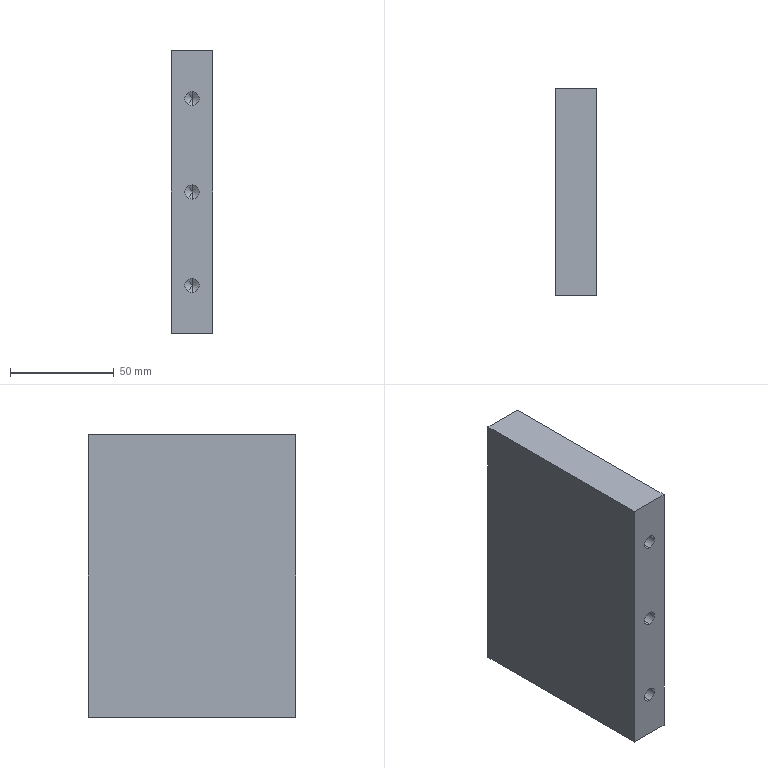Part | SolidWorks | features HoleWzd 2, Extrusion 1 | 1 solid | 30 faces | box 20 x 100 x 136 mm | volume 267548 mm3 | cylinder 12 | cone 12 | plane 6 | commonest cylinder face diameters 6.8 x12
STEP:
#1=CARTESIAN_POINT('',(10.,-30.25,-41.6));
#2=VERTEX_POINT('',#1);
#3=CARTESIAN_POINT('',(10.,-30.25,-48.4));
#4=VERTEX_POINT('',#3);
#5=CARTESIAN_POINT('',(10.,-30.25,-45.));
#6=DIRECTION('',(0.,-1.,0.));
#7=DIRECTION('',(0.,0.,-1.));
#8=AXIS2_PLACEMENT_3D('',#5,#6,#7);
#9=CIRCLE('',#8,3.4);
#10=EDGE_CURVE('',#2,#4,#9,.T.);
#11=ORIENTED_EDGE('',*,*,#10,.F.);
#12=CARTESIAN_POINT('',(10.,-50.,-41.6));
#13=VERTEX_POINT('',#12);
#14=CARTESIAN_POINT('',(10.,-50.,-41.6));
#15=DIRECTION('',(0.,-1.,0.));
#16=VECTOR('',#15,1000.);
#17=LINE('',#14,#16);
#18=EDGE_CURVE('',#2,#13,#17,.T.);
#19=ORIENTED_EDGE('',*,*,#18,.T.);
#20=CARTESIAN_POINT('',(10.,-50.,-48.4));
#21=VERTEX_POINT('',#20);
#22=CARTESIAN_POINT('',(10.,-50.,-45.));
#23=DIRECTION('',(0.,-1.,0.));
#24=DIRECTION('',(0.,0.,-1.));
#25=AXIS2_PLACEMENT_3D('',#22,#23,#24);
#26=CIRCLE('',#25,3.4);
#27=EDGE_CURVE('',#13,#21,#26,.T.);
#28=ORIENTED_EDGE('',*,*,#27,.T.);
#29=CARTESIAN_POINT('',(10.,-50.,-48.4));
#30=DIRECTION('',(0.,-1.,0.));
#31=VECTOR('',#30,1000.);
#32=LINE('',#29,#31);
#33=EDGE_CURVE('',#4,#21,#32,.T.);
#34=ORIENTED_EDGE('',*,*,#33,.F.);
#35=EDGE_LOOP('',(#11,#19,#28,#34));
#36=FACE_OUTER_BOUND('',#35,.T.);
#37=CARTESIAN_POINT('',(10.,-50.,-45.));
#38=DIRECTION('',(0.,-1.,0.));
#39=DIRECTION('',(0.,0.,-1.));
#40=AXIS2_PLACEMENT_3D('',#37,#38,#39);
#41=CYLINDRICAL_SURFACE('',#40,3.4);
#42=ADVANCED_FACE('',(#36),#41,.F.);
#43=CARTESIAN_POINT('',(10.,-28.207,-45.));
#44=VERTEX_POINT('',#43);
#45=CARTESIAN_POINT('',(10.,-30.25,-48.4));
#46=DIRECTION('',(0.,-0.515,-0.8572));
#47=VECTOR('',#46,1000.);
#48=LINE('',#45,#47);
#49=EDGE_CURVE('',#44,#4,#48,.T.);
#50=ORIENTED_EDGE('',*,*,#49,.F.);
#51=CARTESIAN_POINT('',(10.,-30.25,-41.6));
#52=DIRECTION('',(0.,-0.515,0.8572));
#53=VECTOR('',#52,1000.);
#54=LINE('',#51,#53);
#55=EDGE_CURVE('',#44,#2,#54,.T.);
#56=ORIENTED_EDGE('',*,*,#55,.T.);
#57=ORIENTED_EDGE('',*,*,#10,.T.);
#58=EDGE_LOOP('',(#50,#56,#57));
#59=FACE_OUTER_BOUND('',#58,.T.);
#60=CARTESIAN_POINT('',(10.,-30.25,-45.));
#61=DIRECTION('',(0.,-1.,0.));
#62=DIRECTION('',(0.,0.,-1.));
#63=AXIS2_PLACEMENT_3D('',#60,#61,#62);
#64=CONICAL_SURFACE('',#63,3.4,1.03);
#65=ADVANCED_FACE('',(#59),#64,.F.);
#66=CARTESIAN_POINT('',(10.,-30.25,3.4));
#67=VERTEX_POINT('',#66);
#68=CARTESIAN_POINT('',(10.,-30.25,-3.4));
#69=VERTEX_POINT('',#68);
#70=CARTESIAN_POINT('',(10.,-30.25,0.));
#71=DIRECTION('',(0.,-1.,0.));
#72=DIRECTION('',(0.,0.,-1.));
#73=AXIS2_PLACEMENT_3D('',#70,#71,#72);
#74=CIRCLE('',#73,3.4);
#75=EDGE_CURVE('',#67,#69,#74,.T.);
#76=ORIENTED_EDGE('',*,*,#75,.F.);
#77=CARTESIAN_POINT('',(10.,-50.,3.4));
#78=VERTEX_POINT('',#77);
#79=CARTESIAN_POINT('',(10.,-50.,3.4));
#80=DIRECTION('',(0.,-1.,0.));
#81=VECTOR('',#80,1000.);
#82=LINE('',#79,#81);
#83=EDGE_CURVE('',#67,#78,#82,.T.);
#84=ORIENTED_EDGE('',*,*,#83,.T.);
#85=CARTESIAN_POINT('',(10.,-50.,-3.4));
#86=VERTEX_POINT('',#85);
#87=CARTESIAN_POINT('',(10.,-50.,0.));
#88=DIRECTION('',(0.,-1.,0.));
#89=DIRECTION('',(0.,0.,-1.));
#90=AXIS2_PLACEMENT_3D('',#87,#88,#89);
#91=CIRCLE('',#90,3.4);
#92=EDGE_CURVE('',#78,#86,#91,.T.);
#93=ORIENTED_EDGE('',*,*,#92,.T.);
#94=CARTESIAN_POINT('',(10.,-50.,-3.4));
#95=DIRECTION('',(0.,-1.,0.));
#96=VECTOR('',#95,1000.);
#97=LINE('',#94,#96);
#98=EDGE_CURVE('',#69,#86,#97,.T.);
#99=ORIENTED_EDGE('',*,*,#98,.F.);
#100=EDGE_LOOP('',(#76,#84,#93,#99));
#101=FACE_OUTER_BOUND('',#100,.T.);
#102=CARTESIAN_POINT('',(10.,-50.,0.));
#103=DIRECTION('',(0.,-1.,0.));
#104=DIRECTION('',(0.,0.,-1.));
#105=AXIS2_PLACEMENT_3D('',#102,#103,#104);
#106=CYLINDRICAL_SURFACE('',#105,3.4);
#107=ADVANCED_FACE('',(#101),#106,.F.);
#108=CARTESIAN_POINT('',(10.,-28.207,0.));
#109=VERTEX_POINT('',#108);
#110=CARTESIAN_POINT('',(10.,-30.25,-3.4));
#111=DIRECTION('',(0.,-0.515,-0.8572));
#112=VECTOR('',#111,1000.);
#113=LINE('',#110,#112);
#114=EDGE_CURVE('',#109,#69,#113,.T.);
#115=ORIENTED_EDGE('',*,*,#114,.F.);
#116=CARTESIAN_POINT('',(10.,-30.25,3.4));
#117=DIRECTION('',(0.,-0.515,0.8572));
#118=VECTOR('',#117,1000.);
#119=LINE('',#116,#118);
#120=EDGE_CURVE('',#109,#67,#119,.T.);
#121=ORIENTED_EDGE('',*,*,#120,.T.);
#122=ORIENTED_EDGE('',*,*,#75,.T.);
#123=EDGE_LOOP('',(#115,#121,#122));
#124=FACE_OUTER_BOUND('',#123,.T.);
#125=CARTESIAN_POINT('',(10.,-30.25,0.));
#126=DIRECTION('',(0.,-1.,0.));
#127=DIRECTION('',(0.,0.,-1.));
#128=AXIS2_PLACEMENT_3D('',#125,#126,#127);
#129=CONICAL_SURFACE('',#128,3.4,1.03);
#130=ADVANCED_FACE('',(#124),#129,.F.);
#131=CARTESIAN_POINT('',(10.,-30.25,48.4));
#132=VERTEX_POINT('',#131);
#133=CARTESIAN_POINT('',(10.,-30.25,41.6));
#134=VERTEX_POINT('',#133);
#135=CARTESIAN_POINT('',(10.,-30.25,45.));
#136=DIRECTION('',(0.,-1.,0.));
#137=DIRECTION('',(0.,0.,-1.));
#138=AXIS2_PLACEMENT_3D('',#135,#136,#137);
#139=CIRCLE('',#138,3.4);
#140=EDGE_CURVE('',#132,#134,#139,.T.);
#141=ORIENTED_EDGE('',*,*,#140,.F.);
#142=CARTESIAN_POINT('',(10.,-50.,48.4));
#143=VERTEX_POINT('',#142);
#144=CARTESIAN_POINT('',(10.,-50.,48.4));
#145=DIRECTION('',(0.,-1.,0.));
#146=VECTOR('',#145,1000.);
#147=LINE('',#144,#146);
#148=EDGE_CURVE('',#132,#143,#147,.T.);
#149=ORIENTED_EDGE('',*,*,#148,.T.);
#150=CARTESIAN_POINT('',(10.,-50.,41.6));
#151=VERTEX_POINT('',#150);
#152=CARTESIAN_POINT('',(10.,-50.,45.));
#153=DIRECTION('',(0.,-1.,0.));
#154=DIRECTION('',(0.,0.,-1.));
#155=AXIS2_PLACEMENT_3D('',#152,#153,#154);
#156=CIRCLE('',#155,3.4);
#157=EDGE_CURVE('',#143,#151,#156,.T.);
#158=ORIENTED_EDGE('',*,*,#157,.T.);
#159=CARTESIAN_POINT('',(10.,-50.,41.6));
#160=DIRECTION('',(0.,-1.,0.));
#161=VECTOR('',#160,1000.);
#162=LINE('',#159,#161);
#163=EDGE_CURVE('',#134,#151,#162,.T.);
#164=ORIENTED_EDGE('',*,*,#163,.F.);
#165=EDGE_LOOP('',(#141,#149,#158,#164));
#166=FACE_OUTER_BOUND('',#165,.T.);
#167=CARTESIAN_POINT('',(10.,-50.,45.));
#168=DIRECTION('',(0.,-1.,0.));
#169=DIRECTION('',(0.,0.,-1.));
#170=AXIS2_PLACEMENT_3D('',#167,#168,#169);
#171=CYLINDRICAL_SURFACE('',#170,3.4);
#172=ADVANCED_FACE('',(#166),#171,.F.);
#173=CARTESIAN_POINT('',(10.,-28.207,45.));
#174=VERTEX_POINT('',#173);
#175=CARTESIAN_POINT('',(10.,-30.25,41.6));
#176=DIRECTION('',(0.,-0.515,-0.8572));
#177=VECTOR('',#176,1000.);
#178=LINE('',#175,#177);
#179=EDGE_CURVE('',#174,#134,#178,.T.);
#180=ORIENTED_EDGE('',*,*,#179,.F.);
#181=CARTESIAN_POINT('',(10.,-30.25,48.4));
#182=DIRECTION('',(0.,-0.515,0.8572));
#183=VECTOR('',#182,1000.);
#184=LINE('',#181,#183);
#185=EDGE_CURVE('',#174,#132,#184,.T.);
#186=ORIENTED_EDGE('',*,*,#185,.T.);
#187=ORIENTED_EDGE('',*,*,#140,.T.);
#188=EDGE_LOOP('',(#180,#186,#187));
#189=FACE_OUTER_BOUND('',#188,.T.);
#190=CARTESIAN_POINT('',(10.,-30.25,45.));
#191=DIRECTION('',(0.,-1.,0.));
#192=DIRECTION('',(0.,0.,-1.));
#193=AXIS2_PLACEMENT_3D('',#190,#191,#192);
#194=CONICAL_SURFACE('',#193,3.4,1.03);
#195=ADVANCED_FACE('',(#189),#194,.F.);
#196=CARTESIAN_POINT('',(9.91,30.25,-48.4));
#197=VERTEX_POINT('',#196);
#198=CARTESIAN_POINT('',(9.91,30.25,-41.6));
#199=VERTEX_POINT('',#198);
#200=CARTESIAN_POINT('',(9.91,30.25,-45.));
#201=DIRECTION('',(0.,1.,0.));
#202=DIRECTION('',(0.,0.,1.));
#203=AXIS2_PLACEMENT_3D('',#200,#201,#202);
#204=CIRCLE('',#203,3.4);
#205=EDGE_CURVE('',#197,#199,#204,.T.);
#206=ORIENTED_EDGE('',*,*,#205,.F.);
#207=CARTESIAN_POINT('',(9.91,50.,-48.4));
#208=VERTEX_POINT('',#207);
#209=CARTESIAN_POINT('',(9.91,50.,-48.4));
#210=DIRECTION('',(0.,1.,0.));
#211=VECTOR('',#210,1000.);
#212=LINE('',#209,#211);
#213=EDGE_CURVE('',#197,#208,#212,.T.);
#214=ORIENTED_EDGE('',*,*,#213,.T.);
#215=CARTESIAN_POINT('',(9.91,50.,-41.6));
#216=VERTEX_POINT('',#215);
#217=CARTESIAN_POINT('',(9.91,50.,-45.));
#218=DIRECTION('',(0.,1.,0.));
#219=DIRECTION('',(0.,0.,1.));
#220=AXIS2_PLACEMENT_3D('',#217,#218,#219);
#221=CIRCLE('',#220,3.4);
#222=EDGE_CURVE('',#208,#216,#221,.T.);
#223=ORIENTED_EDGE('',*,*,#222,.T.);
#224=CARTESIAN_POINT('',(9.91,50.,-41.6));
#225=DIRECTION('',(0.,1.,0.));
#226=VECTOR('',#225,1000.);
#227=LINE('',#224,#226);
#228=EDGE_CURVE('',#199,#216,#227,.T.);
#229=ORIENTED_EDGE('',*,*,#228,.F.);
#230=EDGE_LOOP('',(#206,#214,#223,#229));
#231=FACE_OUTER_BOUND('',#230,.T.);
#232=CARTESIAN_POINT('',(9.91,50.,-45.));
#233=DIRECTION('',(0.,1.,0.));
#234=DIRECTION('',(0.,0.,1.));
#235=AXIS2_PLACEMENT_3D('',#232,#233,#234);
#236=CYLINDRICAL_SURFACE('',#235,3.4);
#237=ADVANCED_FACE('',(#231),#236,.F.);
#238=CARTESIAN_POINT('',(9.91,28.207,-45.));
#239=VERTEX_POINT('',#238);
#240=CARTESIAN_POINT('',(9.91,30.25,-41.6));
#241=DIRECTION('',(0.,0.515,0.8572));
#242=VECTOR('',#241,1000.);
#243=LINE('',#240,#242);
#244=EDGE_CURVE('',#239,#199,#243,.T.);
#245=ORIENTED_EDGE('',*,*,#244,.F.);
#246=CARTESIAN_POINT('',(9.91,30.25,-48.4));
#247=DIRECTION('',(0.,0.515,-0.8572));
#248=VECTOR('',#247,1000.);
#249=LINE('',#246,#248);
#250=EDGE_CURVE('',#239,#197,#249,.T.);
#251=ORIENTED_EDGE('',*,*,#250,.T.);
#252=ORIENTED_EDGE('',*,*,#205,.T.);
#253=EDGE_LOOP('',(#245,#251,#252));
#254=FACE_OUTER_BOUND('',#253,.T.);
#255=CARTESIAN_POINT('',(9.91,30.25,-45.));
#256=DIRECTION('',(0.,1.,0.));
#257=DIRECTION('',(0.,0.,1.));
#258=AXIS2_PLACEMENT_3D('',#255,#256,#257);
#259=CONICAL_SURFACE('',#258,3.4,1.03);
#260=ADVANCED_FACE('',(#254),#259,.F.);
#261=CARTESIAN_POINT('',(9.91,30.25,41.6));
#262=VERTEX_POINT('',#261);
#263=CARTESIAN_POINT('',(9.91,30.25,48.4));
#264=VERTEX_POINT('',#263);
#265=CARTESIAN_POINT('',(9.91,30.25,45.));
#266=DIRECTION('',(0.,1.,0.));
#267=DIRECTION('',(0.,0.,1.));
#268=AXIS2_PLACEMENT_3D('',#265,#266,#267);
#269=CIRCLE('',#268,3.4);
#270=EDGE_CURVE('',#262,#264,#269,.T.);
#271=ORIENTED_EDGE('',*,*,#270,.F.);
#272=CARTESIAN_POINT('',(9.91,50.,41.6));
#273=VERTEX_POINT('',#272);
#274=CARTESIAN_POINT('',(9.91,50.,41.6));
#275=DIRECTION('',(0.,1.,0.));
#276=VECTOR('',#275,1000.);
#277=LINE('',#274,#276);
#278=EDGE_CURVE('',#262,#273,#277,.T.);
#279=ORIENTED_EDGE('',*,*,#278,.T.);
#280=CARTESIAN_POINT('',(9.91,50.,48.4));
#281=VERTEX_POINT('',#280);
#282=CARTESIAN_POINT('',(9.91,50.,45.));
#283=DIRECTION('',(0.,1.,0.));
#284=DIRECTION('',(0.,0.,1.));
#285=AXIS2_PLACEMENT_3D('',#282,#283,#284);
#286=CIRCLE('',#285,3.4);
#287=EDGE_CURVE('',#273,#281,#286,.T.);
#288=ORIENTED_EDGE('',*,*,#287,.T.);
#289=CARTESIAN_POINT('',(9.91,50.,48.4));
#290=DIRECTION('',(0.,1.,0.));
#291=VECTOR('',#290,1000.);
#292=LINE('',#289,#291);
#293=EDGE_CURVE('',#264,#281,#292,.T.);
#294=ORIENTED_EDGE('',*,*,#293,.F.);
#295=EDGE_LOOP('',(#271,#279,#288,#294));
#296=FACE_OUTER_BOUND('',#295,.T.);
#297=CARTESIAN_POINT('',(9.91,50.,45.));
#298=DIRECTION('',(0.,1.,0.));
#299=DIRECTION('',(0.,0.,1.));
#300=AXIS2_PLACEMENT_3D('',#297,#298,#299);
#301=CYLINDRICAL_SURFACE('',#300,3.4);
#302=ADVANCED_FACE('',(#296),#301,.F.);
#303=CARTESIAN_POINT('',(9.91,28.207,45.));
#304=VERTEX_POINT('',#303);
#305=CARTESIAN_POINT('',(9.91,30.25,48.4));
#306=DIRECTION('',(0.,0.515,0.8572));
#307=VECTOR('',#306,1000.);
#308=LINE('',#305,#307);
#309=EDGE_CURVE('',#304,#264,#308,.T.);
#310=ORIENTED_EDGE('',*,*,#309,.F.);
#311=CARTESIAN_POINT('',(9.91,30.25,41.6));
#312=DIRECTION('',(0.,0.515,-0.8572));
#313=VECTOR('',#312,1000.);
#314=LINE('',#311,#313);
#315=EDGE_CURVE('',#304,#262,#314,.T.);
#316=ORIENTED_EDGE('',*,*,#315,.T.);
#317=ORIENTED_EDGE('',*,*,#270,.T.);
#318=EDGE_LOOP('',(#310,#316,#317));
#319=FACE_OUTER_BOUND('',#318,.T.);
#320=CARTESIAN_POINT('',(9.91,30.25,45.));
#321=DIRECTION('',(0.,1.,0.));
#322=DIRECTION('',(0.,0.,1.));
#323=AXIS2_PLACEMENT_3D('',#320,#321,#322);
#324=CONICAL_SURFACE('',#323,3.4,1.03);
#325=ADVANCED_FACE('',(#319),#324,.F.);
#326=CARTESIAN_POINT('',(9.734,30.25,-3.4));
#327=VERTEX_POINT('',#326);
#328=CARTESIAN_POINT('',(9.734,30.25,3.4));
#329=VERTEX_POINT('',#328);
#330=CARTESIAN_POINT('',(9.734,30.25,0.));
#331=DIRECTION('',(0.,1.,0.));
#332=DIRECTION('',(0.,0.,1.));
#333=AXIS2_PLACEMENT_3D('',#330,#331,#332);
#334=CIRCLE('',#333,3.4);
#335=EDGE_CURVE('',#327,#329,#334,.T.);
#336=ORIENTED_EDGE('',*,*,#335,.F.);
#337=CARTESIAN_POINT('',(9.734,50.,-3.4));
#338=VERTEX_POINT('',#337);
#339=CARTESIAN_POINT('',(9.734,50.,-3.4));
#340=DIRECTION('',(0.,1.,0.));
#341=VECTOR('',#340,1000.);
#342=LINE('',#339,#341);
#343=EDGE_CURVE('',#327,#338,#342,.T.);
#344=ORIENTED_EDGE('',*,*,#343,.T.);
#345=CARTESIAN_POINT('',(9.734,50.,3.4));
#346=VERTEX_POINT('',#345);
#347=CARTESIAN_POINT('',(9.734,50.,0.));
#348=DIRECTION('',(0.,1.,0.));
#349=DIRECTION('',(0.,0.,1.));
#350=AXIS2_PLACEMENT_3D('',#347,#348,#349);
#351=CIRCLE('',#350,3.4);
#352=EDGE_CURVE('',#338,#346,#351,.T.);
#353=ORIENTED_EDGE('',*,*,#352,.T.);
#354=CARTESIAN_POINT('',(9.734,50.,3.4));
#355=DIRECTION('',(0.,1.,0.));
#356=VECTOR('',#355,1000.);
#357=LINE('',#354,#356);
#358=EDGE_CURVE('',#329,#346,#357,.T.);
#359=ORIENTED_EDGE('',*,*,#358,.F.);
#360=EDGE_LOOP('',(#336,#344,#353,#359));
#361=FACE_OUTER_BOUND('',#360,.T.);
#362=CARTESIAN_POINT('',(9.734,50.,0.));
#363=DIRECTION('',(0.,1.,0.));
#364=DIRECTION('',(0.,0.,1.));
#365=AXIS2_PLACEMENT_3D('',#362,#363,#364);
#366=CYLINDRICAL_SURFACE('',#365,3.4);
#367=ADVANCED_FACE('',(#361),#366,.F.);
#368=CARTESIAN_POINT('',(9.734,28.207,0.));
#369=VERTEX_POINT('',#368);
#370=CARTESIAN_POINT('',(9.734,30.25,3.4));
#371=DIRECTION('',(0.,0.515,0.8572));
#372=VECTOR('',#371,1000.);
#373=LINE('',#370,#372);
#374=EDGE_CURVE('',#369,#329,#373,.T.);
#375=ORIENTED_EDGE('',*,*,#374,.F.);
#376=CARTESIAN_POINT('',(9.734,30.25,-3.4));
#377=DIRECTION('',(0.,0.515,-0.8572));
#378=VECTOR('',#377,1000.);
#379=LINE('',#376,#378);
#380=EDGE_CURVE('',#369,#327,#379,.T.);
#381=ORIENTED_EDGE('',*,*,#380,.T.);
#382=ORIENTED_EDGE('',*,*,#335,.T.);
#383=EDGE_LOOP('',(#375,#381,#382));
#384=FACE_OUTER_BOUND('',#383,.T.);
#385=CARTESIAN_POINT('',(9.734,30.25,0.));
#386=DIRECTION('',(0.,1.,0.));
#387=DIRECTION('',(0.,0.,1.));
#388=AXIS2_PLACEMENT_3D('',#385,#386,#387);
#389=CONICAL_SURFACE('',#388,3.4,1.03);
#390=ADVANCED_FACE('',(#384),#389,.F.);
#391=CARTESIAN_POINT('',(0.,-50.,-68.));
#392=VERTEX_POINT('',#391);
#393=CARTESIAN_POINT('',(0.,50.,-68.));
#394=VERTEX_POINT('',#393);
#395=CARTESIAN_POINT('',(0.,50.,-68.));
#396=DIRECTION('',(0.,1.,0.));
#397=VECTOR('',#396,1000.);
#398=LINE('',#395,#397);
#399=EDGE_CURVE('',#392,#394,#398,.T.);
#400=ORIENTED_EDGE('',*,*,#399,.T.);
#401=CARTESIAN_POINT('',(20.,50.,-68.));
#402=VERTEX_POINT('',#401);
#403=CARTESIAN_POINT('',(20.,50.,-68.));
#404=DIRECTION('',(-1.,0.,0.));
#405=VECTOR('',#404,1000.);
#406=LINE('',#403,#405);
#407=EDGE_CURVE('',#402,#394,#406,.T.);
#408=ORIENTED_EDGE('',*,*,#407,.F.);
#409=CARTESIAN_POINT('',(20.,-50.,-68.));
#410=VERTEX_POINT('',#409);
#411=CARTESIAN_POINT('',(20.,50.,-68.));
#412=DIRECTION('',(0.,1.,0.));
#413=VECTOR('',#412,1000.);
#414=LINE('',#411,#413);
#415=EDGE_CURVE('',#410,#402,#414,.T.);
#416=ORIENTED_EDGE('',*,*,#415,.F.);
#417=CARTESIAN_POINT('',(20.,-50.,-68.));
#418=DIRECTION('',(-1.,0.,0.));
#419=VECTOR('',#418,1000.);
#420=LINE('',#417,#419);
#421=EDGE_CURVE('',#410,#392,#420,.T.);
#422=ORIENTED_EDGE('',*,*,#421,.T.);
#423=EDGE_LOOP('',(#400,#408,#416,#422));
#424=FACE_OUTER_BOUND('',#423,.T.);
#425=CARTESIAN_POINT('',(20.,50.,-68.));
#426=DIRECTION('',(0.,0.,1.));
#427=DIRECTION('',(0.,-1.,0.));
#428=AXIS2_PLACEMENT_3D('',#425,#426,#427);
#429=PLANE('',#428);
#430=ADVANCED_FACE('',(#424),#429,.F.);
#431=CARTESIAN_POINT('',(9.91,50.,-45.));
#432=DIRECTION('',(0.,1.,0.));
#433=DIRECTION('',(0.,0.,1.));
#434=AXIS2_PLACEMENT_3D('',#431,#432,#433);
#435=CIRCLE('',#434,3.4);
#436=EDGE_CURVE('',#216,#208,#435,.T.);
#437=ORIENTED_EDGE('',*,*,#436,.F.);
#438=ORIENTED_EDGE('',*,*,#222,.F.);
#439=EDGE_LOOP('',(#437,#438));
#440=FACE_BOUND('',#439,.T.);
#441=CARTESIAN_POINT('',(9.91,50.,45.));
#442=DIRECTION('',(0.,1.,0.));
#443=DIRECTION('',(0.,0.,1.));
#444=AXIS2_PLACEMENT_3D('',#441,#442,#443);
#445=CIRCLE('',#444,3.4);
#446=EDGE_CURVE('',#281,#273,#445,.T.);
#447=ORIENTED_EDGE('',*,*,#446,.F.);
#448=ORIENTED_EDGE('',*,*,#287,.F.);
#449=EDGE_LOOP('',(#447,#448));
#450=FACE_BOUND('',#449,.T.);
#451=CARTESIAN_POINT('',(9.734,50.,0.));
#452=DIRECTION('',(0.,1.,0.));
#453=DIRECTION('',(0.,0.,1.));
#454=AXIS2_PLACEMENT_3D('',#451,#452,#453);
#455=CIRCLE('',#454,3.4);
#456=EDGE_CURVE('',#346,#338,#455,.T.);
#457=ORIENTED_EDGE('',*,*,#456,.F.);
#458=ORIENTED_EDGE('',*,*,#352,.F.);
#459=EDGE_LOOP('',(#457,#458));
#460=FACE_BOUND('',#459,.T.);
#461=CARTESIAN_POINT('',(0.,50.,68.));
#462=VERTEX_POINT('',#461);
#463=CARTESIAN_POINT('',(0.,50.,68.));
#464=DIRECTION('',(0.,0.,1.));
#465=VECTOR('',#464,1000.);
#466=LINE('',#463,#465);
#467=EDGE_CURVE('',#394,#462,#466,.T.);
#468=ORIENTED_EDGE('',*,*,#467,.T.);
#469=CARTESIAN_POINT('',(20.,50.,68.));
#470=VERTEX_POINT('',#469);
#471=CARTESIAN_POINT('',(20.,50.,68.));
#472=DIRECTION('',(-1.,0.,0.));
#473=VECTOR('',#472,1000.);
#474=LINE('',#471,#473);
#475=EDGE_CURVE('',#470,#462,#474,.T.);
#476=ORIENTED_EDGE('',*,*,#475,.F.);
#477=CARTESIAN_POINT('',(20.,50.,68.));
#478=DIRECTION('',(0.,0.,1.));
#479=VECTOR('',#478,1000.);
#480=LINE('',#477,#479);
#481=EDGE_CURVE('',#402,#470,#480,.T.);
#482=ORIENTED_EDGE('',*,*,#481,.F.);
#483=ORIENTED_EDGE('',*,*,#407,.T.);
#484=EDGE_LOOP('',(#468,#476,#482,#483));
#485=FACE_OUTER_BOUND('',#484,.T.);
#486=CARTESIAN_POINT('',(20.,50.,68.));
#487=DIRECTION('',(0.,-1.,0.));
#488=DIRECTION('',(0.,0.,-1.));
#489=AXIS2_PLACEMENT_3D('',#486,#487,#488);
#490=PLANE('',#489);
#491=ADVANCED_FACE('',(#440,#450,#460,#485),#490,.F.);
#492=CARTESIAN_POINT('',(0.,-50.,68.));
#493=VERTEX_POINT('',#492);
#494=CARTESIAN_POINT('',(0.,50.,68.));
#495=DIRECTION('',(0.,-1.,0.));
#496=VECTOR('',#495,1000.);
#497=LINE('',#494,#496);
#498=EDGE_CURVE('',#462,#493,#497,.T.);
#499=ORIENTED_EDGE('',*,*,#498,.T.);
#500=CARTESIAN_POINT('',(20.,-50.,68.));
#501=VERTEX_POINT('',#500);
#502=CARTESIAN_POINT('',(20.,-50.,68.));
#503=DIRECTION('',(-1.,0.,0.));
#504=VECTOR('',#503,1000.);
#505=LINE('',#502,#504);
#506=EDGE_CURVE('',#501,#493,#505,.T.);
#507=ORIENTED_EDGE('',*,*,#506,.F.);
#508=CARTESIAN_POINT('',(20.,50.,68.));
#509=DIRECTION('',(0.,-1.,0.));
#510=VECTOR('',#509,1000.);
#511=LINE('',#508,#510);
#512=EDGE_CURVE('',#470,#501,#511,.T.);
#513=ORIENTED_EDGE('',*,*,#512,.F.);
#514=ORIENTED_EDGE('',*,*,#475,.T.);
#515=EDGE_LOOP('',(#499,#507,#513,#514));
#516=FACE_OUTER_BOUND('',#515,.T.);
#517=CARTESIAN_POINT('',(20.,50.,68.));
#518=DIRECTION('',(0.,0.,-1.));
#519=DIRECTION('',(0.,1.,0.));
#520=AXIS2_PLACEMENT_3D('',#517,#518,#519);
#521=PLANE('',#520);
#522=ADVANCED_FACE('',(#516),#521,.F.);
#523=CARTESIAN_POINT('',(10.,-50.,-45.));
#524=DIRECTION('',(0.,-1.,0.));
#525=DIRECTION('',(0.,0.,-1.));
#526=AXIS2_PLACEMENT_3D('',#523,#524,#525);
#527=CIRCLE('',#526,3.4);
#528=EDGE_CURVE('',#21,#13,#527,.T.);
#529=ORIENTED_EDGE('',*,*,#528,.F.);
#530=ORIENTED_EDGE('',*,*,#27,.F.);
#531=EDGE_LOOP('',(#529,#530));
#532=FACE_BOUND('',#531,.T.);
#533=CARTESIAN_POINT('',(10.,-50.,0.));
#534=DIRECTION('',(0.,-1.,0.));
#535=DIRECTION('',(0.,0.,-1.));
#536=AXIS2_PLACEMENT_3D('',#533,#534,#535);
#537=CIRCLE('',#536,3.4);
#538=EDGE_CURVE('',#86,#78,#537,.T.);
#539=ORIENTED_EDGE('',*,*,#538,.F.);
#540=ORIENTED_EDGE('',*,*,#92,.F.);
#541=EDGE_LOOP('',(#539,#540));
#542=FACE_BOUND('',#541,.T.);
#543=CARTESIAN_POINT('',(10.,-50.,45.));
#544=DIRECTION('',(0.,-1.,0.));
#545=DIRECTION('',(0.,0.,-1.));
#546=AXIS2_PLACEMENT_3D('',#543,#544,#545);
#547=CIRCLE('',#546,3.4);
#548=EDGE_CURVE('',#151,#143,#547,.T.);
#549=ORIENTED_EDGE('',*,*,#548,.F.);
#550=ORIENTED_EDGE('',*,*,#157,.F.);
#551=EDGE_LOOP('',(#549,#550));
#552=FACE_BOUND('',#551,.T.);
#553=CARTESIAN_POINT('',(0.,-50.,68.));
#554=DIRECTION('',(0.,0.,-1.));
#555=VECTOR('',#554,1000.);
#556=LINE('',#553,#555);
#557=EDGE_CURVE('',#493,#392,#556,.T.);
#558=ORIENTED_EDGE('',*,*,#557,.T.);
#559=ORIENTED_EDGE('',*,*,#421,.F.);
#560=CARTESIAN_POINT('',(20.,-50.,68.));
#561=DIRECTION('',(0.,0.,-1.));
#562=VECTOR('',#561,1000.);
#563=LINE('',#560,#562);
#564=EDGE_CURVE('',#501,#410,#563,.T.);
#565=ORIENTED_EDGE('',*,*,#564,.F.);
#566=ORIENTED_EDGE('',*,*,#506,.T.);
#567=EDGE_LOOP('',(#558,#559,#565,#566));
#568=FACE_OUTER_BOUND('',#567,.T.);
#569=CARTESIAN_POINT('',(20.,-50.,68.));
#570=DIRECTION('',(0.,1.,0.));
#571=DIRECTION('',(0.,0.,1.));
#572=AXIS2_PLACEMENT_3D('',#569,#570,#571);
#573=PLANE('',#572);
#574=ADVANCED_FACE('',(#532,#542,#552,#568),#573,.F.);
#575=ORIENTED_EDGE('',*,*,#415,.T.);
#576=ORIENTED_EDGE('',*,*,#481,.T.);
#577=ORIENTED_EDGE('',*,*,#512,.T.);
#578=ORIENTED_EDGE('',*,*,#564,.T.);
#579=EDGE_LOOP('',(#575,#576,#577,#578));
#580=FACE_OUTER_BOUND('',#579,.T.);
#581=CARTESIAN_POINT('',(20.,0.,0.));
#582=DIRECTION('',(1.,0.,0.));
#583=DIRECTION('',(0.,0.,-1.));
#584=AXIS2_PLACEMENT_3D('',#581,#582,#583);
#585=PLANE('',#584);
#586=ADVANCED_FACE('',(#580),#585,.T.);
#587=ORIENTED_EDGE('',*,*,#399,.F.);
#588=ORIENTED_EDGE('',*,*,#557,.F.);
#589=ORIENTED_EDGE('',*,*,#498,.F.);
#590=ORIENTED_EDGE('',*,*,#467,.F.);
#591=EDGE_LOOP('',(#587,#588,#589,#590));
#592=FACE_OUTER_BOUND('',#591,.T.);
#593=CARTESIAN_POINT('',(0.,0.,0.));
#594=DIRECTION('',(1.,0.,0.));
#595=DIRECTION('',(0.,0.,-1.));
#596=AXIS2_PLACEMENT_3D('',#593,#594,#595);
#597=PLANE('',#596);
#598=ADVANCED_FACE('',(#592),#597,.F.);
#599=ORIENTED_EDGE('',*,*,#380,.F.);
#600=ORIENTED_EDGE('',*,*,#374,.T.);
#601=CARTESIAN_POINT('',(9.734,30.25,0.));
#602=DIRECTION('',(0.,1.,0.));
#603=DIRECTION('',(0.,0.,1.));
#604=AXIS2_PLACEMENT_3D('',#601,#602,#603);
#605=CIRCLE('',#604,3.4);
#606=EDGE_CURVE('',#329,#327,#605,.T.);
#607=ORIENTED_EDGE('',*,*,#606,.T.);
#608=EDGE_LOOP('',(#599,#600,#607));
#609=FACE_OUTER_BOUND('',#608,.T.);
#610=CARTESIAN_POINT('',(9.734,30.25,0.));
#611=DIRECTION('',(0.,1.,0.));
#612=DIRECTION('',(0.,0.,1.));
#613=AXIS2_PLACEMENT_3D('',#610,#611,#612);
#614=CONICAL_SURFACE('',#613,3.4,1.03);
#615=ADVANCED_FACE('',(#609),#614,.F.);
#616=ORIENTED_EDGE('',*,*,#343,.F.);
#617=ORIENTED_EDGE('',*,*,#606,.F.);
#618=ORIENTED_EDGE('',*,*,#358,.T.);
#619=ORIENTED_EDGE('',*,*,#456,.T.);
#620=EDGE_LOOP('',(#616,#617,#618,#619));
#621=FACE_OUTER_BOUND('',#620,.T.);
#622=CARTESIAN_POINT('',(9.734,50.,0.));
#623=DIRECTION('',(0.,1.,0.));
#624=DIRECTION('',(0.,0.,1.));
#625=AXIS2_PLACEMENT_3D('',#622,#623,#624);
#626=CYLINDRICAL_SURFACE('',#625,3.4);
#627=ADVANCED_FACE('',(#621),#626,.F.);
#628=ORIENTED_EDGE('',*,*,#315,.F.);
#629=ORIENTED_EDGE('',*,*,#309,.T.);
#630=CARTESIAN_POINT('',(9.91,30.25,45.));
#631=DIRECTION('',(0.,1.,0.));
#632=DIRECTION('',(0.,0.,1.));
#633=AXIS2_PLACEMENT_3D('',#630,#631,#632);
#634=CIRCLE('',#633,3.4);
#635=EDGE_CURVE('',#264,#262,#634,.T.);
#636=ORIENTED_EDGE('',*,*,#635,.T.);
#637=EDGE_LOOP('',(#628,#629,#636));
#638=FACE_OUTER_BOUND('',#637,.T.);
#639=CARTESIAN_POINT('',(9.91,30.25,45.));
#640=DIRECTION('',(0.,1.,0.));
#641=DIRECTION('',(0.,0.,1.));
#642=AXIS2_PLACEMENT_3D('',#639,#640,#641);
#643=CONICAL_SURFACE('',#642,3.4,1.03);
#644=ADVANCED_FACE('',(#638),#643,.F.);
#645=ORIENTED_EDGE('',*,*,#278,.F.);
#646=ORIENTED_EDGE('',*,*,#635,.F.);
#647=ORIENTED_EDGE('',*,*,#293,.T.);
#648=ORIENTED_EDGE('',*,*,#446,.T.);
#649=EDGE_LOOP('',(#645,#646,#647,#648));
#650=FACE_OUTER_BOUND('',#649,.T.);
#651=CARTESIAN_POINT('',(9.91,50.,45.));
#652=DIRECTION('',(0.,1.,0.));
#653=DIRECTION('',(0.,0.,1.));
#654=AXIS2_PLACEMENT_3D('',#651,#652,#653);
#655=CYLINDRICAL_SURFACE('',#654,3.4);
#656=ADVANCED_FACE('',(#650),#655,.F.);
#657=ORIENTED_EDGE('',*,*,#250,.F.);
#658=ORIENTED_EDGE('',*,*,#244,.T.);
#659=CARTESIAN_POINT('',(9.91,30.25,-45.));
#660=DIRECTION('',(0.,1.,0.));
#661=DIRECTION('',(0.,0.,1.));
#662=AXIS2_PLACEMENT_3D('',#659,#660,#661);
#663=CIRCLE('',#662,3.4);
#664=EDGE_CURVE('',#199,#197,#663,.T.);
#665=ORIENTED_EDGE('',*,*,#664,.T.);
#666=EDGE_LOOP('',(#657,#658,#665));
#667=FACE_OUTER_BOUND('',#666,.T.);
#668=CARTESIAN_POINT('',(9.91,30.25,-45.));
#669=DIRECTION('',(0.,1.,0.));
#670=DIRECTION('',(0.,0.,1.));
#671=AXIS2_PLACEMENT_3D('',#668,#669,#670);
#672=CONICAL_SURFACE('',#671,3.4,1.03);
#673=ADVANCED_FACE('',(#667),#672,.F.);
#674=ORIENTED_EDGE('',*,*,#213,.F.);
#675=ORIENTED_EDGE('',*,*,#664,.F.);
#676=ORIENTED_EDGE('',*,*,#228,.T.);
#677=ORIENTED_EDGE('',*,*,#436,.T.);
#678=EDGE_LOOP('',(#674,#675,#676,#677));
#679=FACE_OUTER_BOUND('',#678,.T.);
#680=CARTESIAN_POINT('',(9.91,50.,-45.));
#681=DIRECTION('',(0.,1.,0.));
#682=DIRECTION('',(0.,0.,1.));
#683=AXIS2_PLACEMENT_3D('',#680,#681,#682);
#684=CYLINDRICAL_SURFACE('',#683,3.4);
#685=ADVANCED_FACE('',(#679),#684,.F.);
#686=ORIENTED_EDGE('',*,*,#185,.F.);
#687=ORIENTED_EDGE('',*,*,#179,.T.);
#688=CARTESIAN_POINT('',(10.,-30.25,45.));
#689=DIRECTION('',(0.,-1.,0.));
#690=DIRECTION('',(0.,0.,-1.));
#691=AXIS2_PLACEMENT_3D('',#688,#689,#690);
#692=CIRCLE('',#691,3.4);
#693=EDGE_CURVE('',#134,#132,#692,.T.);
#694=ORIENTED_EDGE('',*,*,#693,.T.);
#695=EDGE_LOOP('',(#686,#687,#694));
#696=FACE_OUTER_BOUND('',#695,.T.);
#697=CARTESIAN_POINT('',(10.,-30.25,45.));
#698=DIRECTION('',(0.,-1.,0.));
#699=DIRECTION('',(0.,0.,-1.));
#700=AXIS2_PLACEMENT_3D('',#697,#698,#699);
#701=CONICAL_SURFACE('',#700,3.4,1.03);
#702=ADVANCED_FACE('',(#696),#701,.F.);
#703=ORIENTED_EDGE('',*,*,#148,.F.);
#704=ORIENTED_EDGE('',*,*,#693,.F.);
#705=ORIENTED_EDGE('',*,*,#163,.T.);
#706=ORIENTED_EDGE('',*,*,#548,.T.);
#707=EDGE_LOOP('',(#703,#704,#705,#706));
#708=FACE_OUTER_BOUND('',#707,.T.);
#709=CARTESIAN_POINT('',(10.,-50.,45.));
#710=DIRECTION('',(0.,-1.,0.));
#711=DIRECTION('',(0.,0.,-1.));
#712=AXIS2_PLACEMENT_3D('',#709,#710,#711);
#713=CYLINDRICAL_SURFACE('',#712,3.4);
#714=ADVANCED_FACE('',(#708),#713,.F.);
#715=ORIENTED_EDGE('',*,*,#120,.F.);
#716=ORIENTED_EDGE('',*,*,#114,.T.);
#717=CARTESIAN_POINT('',(10.,-30.25,0.));
#718=DIRECTION('',(0.,-1.,0.));
#719=DIRECTION('',(0.,0.,-1.));
#720=AXIS2_PLACEMENT_3D('',#717,#718,#719);
#721=CIRCLE('',#720,3.4);
#722=EDGE_CURVE('',#69,#67,#721,.T.);
#723=ORIENTED_EDGE('',*,*,#722,.T.);
#724=EDGE_LOOP('',(#715,#716,#723));
#725=FACE_OUTER_BOUND('',#724,.T.);
#726=CARTESIAN_POINT('',(10.,-30.25,0.));
#727=DIRECTION('',(0.,-1.,0.));
#728=DIRECTION('',(0.,0.,-1.));
#729=AXIS2_PLACEMENT_3D('',#726,#727,#728);
#730=CONICAL_SURFACE('',#729,3.4,1.03);
#731=ADVANCED_FACE('',(#725),#730,.F.);
#732=ORIENTED_EDGE('',*,*,#83,.F.);
#733=ORIENTED_EDGE('',*,*,#722,.F.);
#734=ORIENTED_EDGE('',*,*,#98,.T.);
#735=ORIENTED_EDGE('',*,*,#538,.T.);
#736=EDGE_LOOP('',(#732,#733,#734,#735));
#737=FACE_OUTER_BOUND('',#736,.T.);
#738=CARTESIAN_POINT('',(10.,-50.,0.));
#739=DIRECTION('',(0.,-1.,0.));
#740=DIRECTION('',(0.,0.,-1.));
#741=AXIS2_PLACEMENT_3D('',#738,#739,#740);
#742=CYLINDRICAL_SURFACE('',#741,3.4);
#743=ADVANCED_FACE('',(#737),#742,.F.);
#744=ORIENTED_EDGE('',*,*,#55,.F.);
#745=ORIENTED_EDGE('',*,*,#49,.T.);
#746=CARTESIAN_POINT('',(10.,-30.25,-45.));
#747=DIRECTION('',(0.,-1.,0.));
#748=DIRECTION('',(0.,0.,-1.));
#749=AXIS2_PLACEMENT_3D('',#746,#747,#748);
#750=CIRCLE('',#749,3.4);
#751=EDGE_CURVE('',#4,#2,#750,.T.);
#752=ORIENTED_EDGE('',*,*,#751,.T.);
#753=EDGE_LOOP('',(#744,#745,#752));
#754=FACE_OUTER_BOUND('',#753,.T.);
#755=CARTESIAN_POINT('',(10.,-30.25,-45.));
#756=DIRECTION('',(0.,-1.,0.));
#757=DIRECTION('',(0.,0.,-1.));
#758=AXIS2_PLACEMENT_3D('',#755,#756,#757);
#759=CONICAL_SURFACE('',#758,3.4,1.03);
#760=ADVANCED_FACE('',(#754),#759,.F.);
#761=ORIENTED_EDGE('',*,*,#18,.F.);
#762=ORIENTED_EDGE('',*,*,#751,.F.);
#763=ORIENTED_EDGE('',*,*,#33,.T.);
#764=ORIENTED_EDGE('',*,*,#528,.T.);
#765=EDGE_LOOP('',(#761,#762,#763,#764));
#766=FACE_OUTER_BOUND('',#765,.T.);
#767=CARTESIAN_POINT('',(10.,-50.,-45.));
#768=DIRECTION('',(0.,-1.,0.));
#769=DIRECTION('',(0.,0.,-1.));
#770=AXIS2_PLACEMENT_3D('',#767,#768,#769);
#771=CYLINDRICAL_SURFACE('',#770,3.4);
#772=ADVANCED_FACE('',(#766),#771,.F.);
#773=CLOSED_SHELL('',(#42,#65,#107,#130,#172,#195,#237,#260,#302,#325,#367,#390,#430,#491,#522,#574,#586,#598,#615,#627,#644,#656,#673,#685,#702,#714,#731,#743,#760,#772));
#774=MANIFOLD_SOLID_BREP('',#773);
#775=CARTESIAN_POINT('',(0.,0.,0.));
#776=DIRECTION('',(0.,0.,1.));
#777=DIRECTION('',(1.,0.,0.));
#778=AXIS2_PLACEMENT_3D('',#775,#776,#777);
#779=(LENGTH_UNIT()NAMED_UNIT(*)SI_UNIT(.MILLI.,.METRE.));
#780=UNCERTAINTY_MEASURE_WITH_UNIT(LENGTH_MEASURE(0.00001),#779,'','');
#781=(NAMED_UNIT(*)PLANE_ANGLE_UNIT()SI_UNIT($,.RADIAN.));
#782=(NAMED_UNIT(*)SI_UNIT($,.STERADIAN.)SOLID_ANGLE_UNIT());
#783=(GEOMETRIC_REPRESENTATION_CONTEXT(3)GLOBAL_UNCERTAINTY_ASSIGNED_CONTEXT((#780))GLOBAL_UNIT_ASSIGNED_CONTEXT((#779,#781,#782))REPRESENTATION_CONTEXT('',''));
#784=ADVANCED_BREP_SHAPE_REPRESENTATION('',(#774,#778),#783);